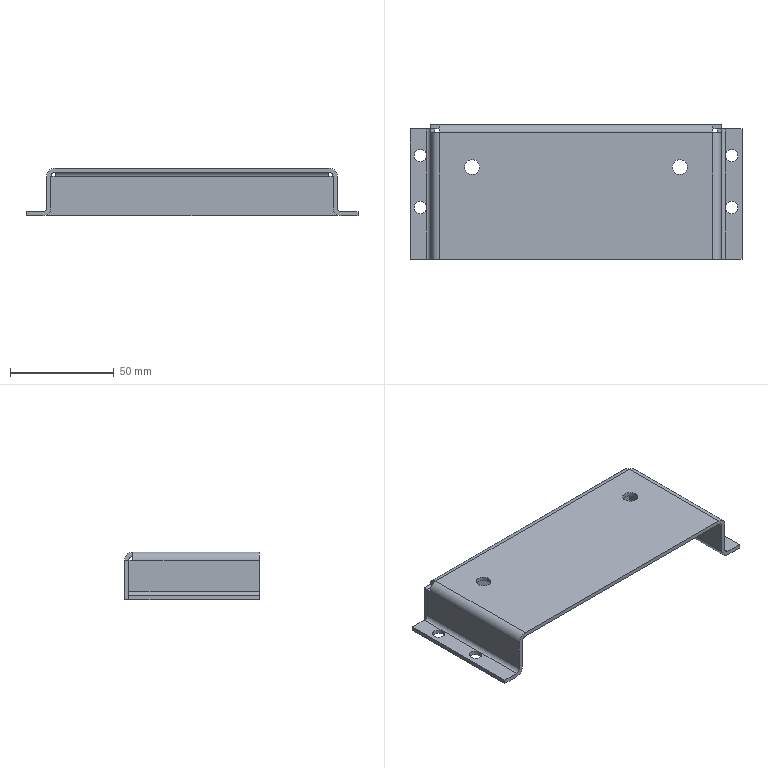Part | NX | features solid 2 | 1 solid | 50 faces | box 160 x 65 x 23 mm | volume 30401 mm3 | plane 28 | cylinder 22 | commonest cylinder face diameters 6 x8 4 x5 8 x5 7.2 x4
STEP:
#1=CARTESIAN_POINT('',(-346.,-1503.,1272.));
#2=VERTEX_POINT('',#1);
#3=CARTESIAN_POINT('',(-346.,-1503.,1274.));
#4=VERTEX_POINT('',#3);
#5=CARTESIAN_POINT('',(-346.,-1503.,1120.776));
#6=DIRECTION('',(0.,0.,1.));
#7=VECTOR('',#6,1000.);
#8=LINE('',#5,#7);
#9=EDGE_CURVE('',#2,#4,#8,.T.);
#10=ORIENTED_EDGE('',*,*,#9,.F.);
#11=CARTESIAN_POINT('',(-352.,-1503.,1272.));
#12=VERTEX_POINT('',#11);
#13=CARTESIAN_POINT('',(-349.,-1503.,1272.));
#14=DIRECTION('',(0.,0.,-1.));
#15=DIRECTION('',(1.,0.,0.));
#16=AXIS2_PLACEMENT_3D('',#13,#14,#15);
#17=CIRCLE('',#16,3.);
#18=EDGE_CURVE('',#2,#12,#17,.T.);
#19=ORIENTED_EDGE('',*,*,#18,.T.);
#20=CARTESIAN_POINT('',(-352.,-1503.,1274.));
#21=VERTEX_POINT('',#20);
#22=CARTESIAN_POINT('',(-352.,-1503.,1120.776));
#23=DIRECTION('',(0.,0.,1.));
#24=VECTOR('',#23,1000.);
#25=LINE('',#22,#24);
#26=EDGE_CURVE('',#21,#12,#25,.F.);
#27=ORIENTED_EDGE('',*,*,#26,.F.);
#28=CARTESIAN_POINT('',(-349.,-1503.,1274.));
#29=DIRECTION('',(0.,0.,-1.));
#30=DIRECTION('',(1.,0.,0.));
#31=AXIS2_PLACEMENT_3D('',#28,#29,#30);
#32=CIRCLE('',#31,3.);
#33=EDGE_CURVE('',#4,#21,#32,.T.);
#34=ORIENTED_EDGE('',*,*,#33,.F.);
#35=EDGE_LOOP('',(#10,#19,#27,#34));
#36=FACE_BOUND('',#35,.T.);
#37=CARTESIAN_POINT('',(-349.,-1503.,1120.776));
#38=DIRECTION('',(0.,0.,1.));
#39=DIRECTION('',(-1.,0.,0.));
#40=AXIS2_PLACEMENT_3D('',#37,#38,#39);
#41=CYLINDRICAL_SURFACE('',#40,3.);
#42=ADVANCED_FACE('',(#36),#41,.F.);
#43=CARTESIAN_POINT('',(-346.,-1528.,1274.));
#44=VERTEX_POINT('',#43);
#45=CARTESIAN_POINT('',(-346.,-1528.,1272.));
#46=VERTEX_POINT('',#45);
#47=CARTESIAN_POINT('',(-346.,-1528.,1120.776));
#48=DIRECTION('',(0.,0.,1.));
#49=VECTOR('',#48,1000.);
#50=LINE('',#47,#49);
#51=EDGE_CURVE('',#44,#46,#50,.F.);
#52=ORIENTED_EDGE('',*,*,#51,.T.);
#53=CARTESIAN_POINT('',(-352.,-1528.,1272.));
#54=VERTEX_POINT('',#53);
#55=CARTESIAN_POINT('',(-349.,-1528.,1272.));
#56=DIRECTION('',(0.,0.,-1.));
#57=DIRECTION('',(1.,0.,0.));
#58=AXIS2_PLACEMENT_3D('',#55,#56,#57);
#59=CIRCLE('',#58,3.);
#60=EDGE_CURVE('',#46,#54,#59,.T.);
#61=ORIENTED_EDGE('',*,*,#60,.T.);
#62=CARTESIAN_POINT('',(-352.,-1528.,1274.));
#63=VERTEX_POINT('',#62);
#64=CARTESIAN_POINT('',(-352.,-1528.,1120.776));
#65=DIRECTION('',(0.,0.,1.));
#66=VECTOR('',#65,1000.);
#67=LINE('',#64,#66);
#68=EDGE_CURVE('',#54,#63,#67,.T.);
#69=ORIENTED_EDGE('',*,*,#68,.T.);
#70=CARTESIAN_POINT('',(-349.,-1528.,1274.));
#71=DIRECTION('',(0.,0.,-1.));
#72=DIRECTION('',(1.,0.,0.));
#73=AXIS2_PLACEMENT_3D('',#70,#71,#72);
#74=CIRCLE('',#73,3.);
#75=EDGE_CURVE('',#44,#63,#74,.T.);
#76=ORIENTED_EDGE('',*,*,#75,.F.);
#77=EDGE_LOOP('',(#52,#61,#69,#76));
#78=FACE_BOUND('',#77,.T.);
#79=CARTESIAN_POINT('',(-349.,-1528.,1120.776));
#80=DIRECTION('',(0.,0.,1.));
#81=DIRECTION('',(-1.,0.,0.));
#82=AXIS2_PLACEMENT_3D('',#79,#80,#81);
#83=CYLINDRICAL_SURFACE('',#82,3.);
#84=ADVANCED_FACE('',(#78),#83,.F.);
#85=CARTESIAN_POINT('',(-496.,-1528.,1272.));
#86=VERTEX_POINT('',#85);
#87=CARTESIAN_POINT('',(-496.,-1528.,1274.));
#88=VERTEX_POINT('',#87);
#89=CARTESIAN_POINT('',(-496.,-1528.,1120.776));
#90=DIRECTION('',(0.,0.,1.));
#91=VECTOR('',#90,1000.);
#92=LINE('',#89,#91);
#93=EDGE_CURVE('',#86,#88,#92,.T.);
#94=ORIENTED_EDGE('',*,*,#93,.F.);
#95=CARTESIAN_POINT('',(-502.,-1528.,1272.));
#96=VERTEX_POINT('',#95);
#97=CARTESIAN_POINT('',(-499.,-1528.,1272.));
#98=DIRECTION('',(0.,0.,-1.));
#99=DIRECTION('',(1.,0.,0.));
#100=AXIS2_PLACEMENT_3D('',#97,#98,#99);
#101=CIRCLE('',#100,3.);
#102=EDGE_CURVE('',#86,#96,#101,.T.);
#103=ORIENTED_EDGE('',*,*,#102,.T.);
#104=CARTESIAN_POINT('',(-502.,-1528.,1274.));
#105=VERTEX_POINT('',#104);
#106=CARTESIAN_POINT('',(-502.,-1528.,1120.776));
#107=DIRECTION('',(0.,0.,1.));
#108=VECTOR('',#107,1000.);
#109=LINE('',#106,#108);
#110=EDGE_CURVE('',#105,#96,#109,.F.);
#111=ORIENTED_EDGE('',*,*,#110,.F.);
#112=CARTESIAN_POINT('',(-499.,-1528.,1274.));
#113=DIRECTION('',(0.,0.,-1.));
#114=DIRECTION('',(1.,0.,0.));
#115=AXIS2_PLACEMENT_3D('',#112,#113,#114);
#116=CIRCLE('',#115,3.);
#117=EDGE_CURVE('',#88,#105,#116,.T.);
#118=ORIENTED_EDGE('',*,*,#117,.F.);
#119=EDGE_LOOP('',(#94,#103,#111,#118));
#120=FACE_BOUND('',#119,.T.);
#121=CARTESIAN_POINT('',(-499.,-1528.,1120.776));
#122=DIRECTION('',(0.,0.,1.));
#123=DIRECTION('',(-1.,0.,0.));
#124=AXIS2_PLACEMENT_3D('',#121,#122,#123);
#125=CYLINDRICAL_SURFACE('',#124,3.);
#126=ADVANCED_FACE('',(#120),#125,.F.);
#127=CARTESIAN_POINT('',(-496.,-1503.,1274.));
#128=VERTEX_POINT('',#127);
#129=CARTESIAN_POINT('',(-496.,-1503.,1272.));
#130=VERTEX_POINT('',#129);
#131=CARTESIAN_POINT('',(-496.,-1503.,1120.776));
#132=DIRECTION('',(0.,0.,1.));
#133=VECTOR('',#132,1000.);
#134=LINE('',#131,#133);
#135=EDGE_CURVE('',#128,#130,#134,.F.);
#136=ORIENTED_EDGE('',*,*,#135,.T.);
#137=CARTESIAN_POINT('',(-502.,-1503.,1272.));
#138=VERTEX_POINT('',#137);
#139=CARTESIAN_POINT('',(-499.,-1503.,1272.));
#140=DIRECTION('',(0.,0.,-1.));
#141=DIRECTION('',(1.,0.,0.));
#142=AXIS2_PLACEMENT_3D('',#139,#140,#141);
#143=CIRCLE('',#142,3.);
#144=EDGE_CURVE('',#130,#138,#143,.T.);
#145=ORIENTED_EDGE('',*,*,#144,.T.);
#146=CARTESIAN_POINT('',(-502.,-1503.,1274.));
#147=VERTEX_POINT('',#146);
#148=CARTESIAN_POINT('',(-502.,-1503.,1120.776));
#149=DIRECTION('',(0.,0.,1.));
#150=VECTOR('',#149,1000.);
#151=LINE('',#148,#150);
#152=EDGE_CURVE('',#138,#147,#151,.T.);
#153=ORIENTED_EDGE('',*,*,#152,.T.);
#154=CARTESIAN_POINT('',(-499.,-1503.,1274.));
#155=DIRECTION('',(0.,0.,-1.));
#156=DIRECTION('',(1.,0.,0.));
#157=AXIS2_PLACEMENT_3D('',#154,#155,#156);
#158=CIRCLE('',#157,3.);
#159=EDGE_CURVE('',#128,#147,#158,.T.);
#160=ORIENTED_EDGE('',*,*,#159,.F.);
#161=EDGE_LOOP('',(#136,#145,#153,#160));
#162=FACE_BOUND('',#161,.T.);
#163=CARTESIAN_POINT('',(-499.,-1503.,1120.776));
#164=DIRECTION('',(0.,0.,1.));
#165=DIRECTION('',(-1.,0.,0.));
#166=AXIS2_PLACEMENT_3D('',#163,#164,#165);
#167=CYLINDRICAL_SURFACE('',#166,3.);
#168=ADVANCED_FACE('',(#162),#167,.F.);
#169=CARTESIAN_POINT('',(-494.,-1553.,1276.));
#170=VERTEX_POINT('',#169);
#171=CARTESIAN_POINT('',(-494.,-1490.1,1276.));
#172=VERTEX_POINT('',#171);
#173=CARTESIAN_POINT('',(-494.,-1553.,1276.));
#174=DIRECTION('',(0.,1.,0.));
#175=VECTOR('',#174,1000.);
#176=LINE('',#173,#175);
#177=EDGE_CURVE('',#170,#172,#176,.T.);
#178=ORIENTED_EDGE('',*,*,#177,.T.);
#179=CARTESIAN_POINT('',(-496.,-1490.1,1274.));
#180=VERTEX_POINT('',#179);
#181=CARTESIAN_POINT('',(-496.,-1490.1,1276.));
#182=DIRECTION('',(0.,1.,0.));
#183=DIRECTION('',(0.,0.,-1.));
#184=AXIS2_PLACEMENT_3D('',#181,#182,#183);
#185=CIRCLE('',#184,2.);
#186=EDGE_CURVE('',#172,#180,#185,.T.);
#187=ORIENTED_EDGE('',*,*,#186,.T.);
#188=CARTESIAN_POINT('',(-496.,-1490.1,1274.));
#189=DIRECTION('',(0.,-1.,0.));
#190=VECTOR('',#189,1000.);
#191=LINE('',#188,#190);
#192=EDGE_CURVE('',#180,#128,#191,.T.);
#193=ORIENTED_EDGE('',*,*,#192,.T.);
#194=CARTESIAN_POINT('',(-496.,-1490.1,1274.));
#195=DIRECTION('',(0.,-1.,0.));
#196=VECTOR('',#195,1000.);
#197=LINE('',#194,#196);
#198=EDGE_CURVE('',#128,#88,#197,.T.);
#199=ORIENTED_EDGE('',*,*,#198,.T.);
#200=CARTESIAN_POINT('',(-496.,-1553.,1274.));
#201=VERTEX_POINT('',#200);
#202=CARTESIAN_POINT('',(-496.,-1490.1,1274.));
#203=DIRECTION('',(0.,-1.,0.));
#204=VECTOR('',#203,1000.);
#205=LINE('',#202,#204);
#206=EDGE_CURVE('',#88,#201,#205,.T.);
#207=ORIENTED_EDGE('',*,*,#206,.T.);
#208=CARTESIAN_POINT('',(-496.,-1553.,1276.));
#209=DIRECTION('',(0.,1.,0.));
#210=DIRECTION('',(0.,0.,-1.));
#211=AXIS2_PLACEMENT_3D('',#208,#209,#210);
#212=CIRCLE('',#211,2.);
#213=EDGE_CURVE('',#170,#201,#212,.T.);
#214=ORIENTED_EDGE('',*,*,#213,.F.);
#215=EDGE_LOOP('',(#178,#187,#193,#199,#207,#214));
#216=FACE_BOUND('',#215,.T.);
#217=CARTESIAN_POINT('',(-496.,-1553.,1276.));
#218=DIRECTION('',(0.,1.,0.));
#219=DIRECTION('',(-1.,0.,0.));
#220=AXIS2_PLACEMENT_3D('',#217,#218,#219);
#221=CYLINDRICAL_SURFACE('',#220,2.);
#222=ADVANCED_FACE('',(#216),#221,.F.);
#223=CARTESIAN_POINT('',(-492.,-1553.,1276.));
#224=VERTEX_POINT('',#223);
#225=CARTESIAN_POINT('',(-492.,-1490.1,1276.));
#226=VERTEX_POINT('',#225);
#227=CARTESIAN_POINT('',(-492.,-1553.,1276.));
#228=DIRECTION('',(0.,1.,0.));
#229=VECTOR('',#228,1000.);
#230=LINE('',#227,#229);
#231=EDGE_CURVE('',#224,#226,#230,.T.);
#232=ORIENTED_EDGE('',*,*,#231,.F.);
#233=CARTESIAN_POINT('',(-496.,-1553.,1272.));
#234=VERTEX_POINT('',#233);
#235=CARTESIAN_POINT('',(-496.,-1553.,1276.));
#236=DIRECTION('',(0.,1.,0.));
#237=DIRECTION('',(-1.,0.,0.));
#238=AXIS2_PLACEMENT_3D('',#235,#236,#237);
#239=CIRCLE('',#238,4.);
#240=EDGE_CURVE('',#224,#234,#239,.T.);
#241=ORIENTED_EDGE('',*,*,#240,.T.);
#242=CARTESIAN_POINT('',(-496.,-1490.1,1272.));
#243=DIRECTION('',(0.,-1.,0.));
#244=VECTOR('',#243,1000.);
#245=LINE('',#242,#244);
#246=EDGE_CURVE('',#86,#234,#245,.T.);
#247=ORIENTED_EDGE('',*,*,#246,.F.);
#248=CARTESIAN_POINT('',(-496.,-1490.1,1272.));
#249=DIRECTION('',(0.,-1.,0.));
#250=VECTOR('',#249,1000.);
#251=LINE('',#248,#250);
#252=EDGE_CURVE('',#130,#86,#251,.T.);
#253=ORIENTED_EDGE('',*,*,#252,.F.);
#254=CARTESIAN_POINT('',(-496.,-1490.1,1272.));
#255=VERTEX_POINT('',#254);
#256=CARTESIAN_POINT('',(-496.,-1490.1,1272.));
#257=DIRECTION('',(0.,-1.,0.));
#258=VECTOR('',#257,1000.);
#259=LINE('',#256,#258);
#260=EDGE_CURVE('',#255,#130,#259,.T.);
#261=ORIENTED_EDGE('',*,*,#260,.F.);
#262=CARTESIAN_POINT('',(-496.,-1490.1,1276.));
#263=DIRECTION('',(0.,1.,0.));
#264=DIRECTION('',(-1.,0.,0.));
#265=AXIS2_PLACEMENT_3D('',#262,#263,#264);
#266=CIRCLE('',#265,4.);
#267=EDGE_CURVE('',#226,#255,#266,.T.);
#268=ORIENTED_EDGE('',*,*,#267,.F.);
#269=EDGE_LOOP('',(#232,#241,#247,#253,#261,#268));
#270=FACE_BOUND('',#269,.T.);
#271=CARTESIAN_POINT('',(-496.,-1553.,1276.));
#272=DIRECTION('',(0.,1.,0.));
#273=DIRECTION('',(-1.,0.,0.));
#274=AXIS2_PLACEMENT_3D('',#271,#272,#273);
#275=CYLINDRICAL_SURFACE('',#274,4.);
#276=ADVANCED_FACE('',(#270),#275,.T.);
#277=CARTESIAN_POINT('',(-504.,-1553.,1274.));
#278=VERTEX_POINT('',#277);
#279=CARTESIAN_POINT('',(-504.,-1490.1,1274.));
#280=VERTEX_POINT('',#279);
#281=CARTESIAN_POINT('',(-504.,-1553.,1274.));
#282=DIRECTION('',(0.,1.,0.));
#283=VECTOR('',#282,1000.);
#284=LINE('',#281,#283);
#285=EDGE_CURVE('',#278,#280,#284,.T.);
#286=ORIENTED_EDGE('',*,*,#285,.T.);
#287=CARTESIAN_POINT('',(-504.,-1490.1,1272.));
#288=VERTEX_POINT('',#287);
#289=CARTESIAN_POINT('',(-504.,-1490.1,1272.));
#290=DIRECTION('',(0.,0.,1.));
#291=VECTOR('',#290,1000.);
#292=LINE('',#289,#291);
#293=EDGE_CURVE('',#288,#280,#292,.T.);
#294=ORIENTED_EDGE('',*,*,#293,.F.);
#295=CARTESIAN_POINT('',(-504.,-1553.,1272.));
#296=VERTEX_POINT('',#295);
#297=CARTESIAN_POINT('',(-504.,-1553.,1272.));
#298=DIRECTION('',(0.,1.,0.));
#299=VECTOR('',#298,1000.);
#300=LINE('',#297,#299);
#301=EDGE_CURVE('',#296,#288,#300,.T.);
#302=ORIENTED_EDGE('',*,*,#301,.F.);
#303=CARTESIAN_POINT('',(-504.,-1553.,1272.));
#304=DIRECTION('',(0.,0.,1.));
#305=VECTOR('',#304,1000.);
#306=LINE('',#303,#305);
#307=EDGE_CURVE('',#296,#278,#306,.T.);
#308=ORIENTED_EDGE('',*,*,#307,.T.);
#309=EDGE_LOOP('',(#286,#294,#302,#308));
#310=FACE_BOUND('',#309,.T.);
#311=CARTESIAN_POINT('',(-504.,-1553.,1272.));
#312=DIRECTION('',(1.,0.,0.));
#313=DIRECTION('',(0.,0.,-1.));
#314=AXIS2_PLACEMENT_3D('',#311,#312,#313);
#315=PLANE('',#314);
#316=ADVANCED_FACE('',(#310),#315,.F.);
#317=ORIENTED_EDGE('',*,*,#206,.F.);
#318=ORIENTED_EDGE('',*,*,#117,.T.);
#319=CARTESIAN_POINT('',(-499.,-1528.,1274.));
#320=DIRECTION('',(0.,0.,-1.));
#321=DIRECTION('',(1.,0.,0.));
#322=AXIS2_PLACEMENT_3D('',#319,#320,#321);
#323=CIRCLE('',#322,3.);
#324=EDGE_CURVE('',#105,#88,#323,.T.);
#325=ORIENTED_EDGE('',*,*,#324,.T.);
#326=ORIENTED_EDGE('',*,*,#198,.F.);
#327=ORIENTED_EDGE('',*,*,#159,.T.);
#328=CARTESIAN_POINT('',(-499.,-1503.,1274.));
#329=DIRECTION('',(0.,0.,-1.));
#330=DIRECTION('',(1.,0.,0.));
#331=AXIS2_PLACEMENT_3D('',#328,#329,#330);
#332=CIRCLE('',#331,3.);
#333=EDGE_CURVE('',#147,#128,#332,.T.);
#334=ORIENTED_EDGE('',*,*,#333,.T.);
#335=ORIENTED_EDGE('',*,*,#192,.F.);
#336=CARTESIAN_POINT('',(-493.722,-1490.1,1274.));
#337=DIRECTION('',(1.,0.,0.));
#338=VECTOR('',#337,1000.);
#339=LINE('',#336,#338);
#340=EDGE_CURVE('',#280,#180,#339,.T.);
#341=ORIENTED_EDGE('',*,*,#340,.F.);
#342=ORIENTED_EDGE('',*,*,#285,.F.);
#343=CARTESIAN_POINT('',(-493.722,-1553.,1274.));
#344=DIRECTION('',(-1.,0.,0.));
#345=VECTOR('',#344,1000.);
#346=LINE('',#343,#345);
#347=EDGE_CURVE('',#201,#278,#346,.T.);
#348=ORIENTED_EDGE('',*,*,#347,.F.);
#349=EDGE_LOOP('',(#317,#318,#325,#326,#327,#334,#335,#341,#342,#348));
#350=FACE_BOUND('',#349,.T.);
#351=CARTESIAN_POINT('',(-1166.5,-2145.,1274.));
#352=DIRECTION('',(0.,0.,-1.));
#353=DIRECTION('',(-1.,0.,0.));
#354=AXIS2_PLACEMENT_3D('',#351,#352,#353);
#355=PLANE('',#354);
#356=ADVANCED_FACE('',(#350),#355,.F.);
#357=ORIENTED_EDGE('',*,*,#252,.T.);
#358=CARTESIAN_POINT('',(-499.,-1528.,1272.));
#359=DIRECTION('',(0.,0.,-1.));
#360=DIRECTION('',(1.,0.,0.));
#361=AXIS2_PLACEMENT_3D('',#358,#359,#360);
#362=CIRCLE('',#361,3.);
#363=EDGE_CURVE('',#96,#86,#362,.T.);
#364=ORIENTED_EDGE('',*,*,#363,.F.);
#365=ORIENTED_EDGE('',*,*,#102,.F.);
#366=ORIENTED_EDGE('',*,*,#246,.T.);
#367=CARTESIAN_POINT('',(-493.722,-1553.,1272.));
#368=DIRECTION('',(-1.,0.,0.));
#369=VECTOR('',#368,1000.);
#370=LINE('',#367,#369);
#371=EDGE_CURVE('',#234,#296,#370,.T.);
#372=ORIENTED_EDGE('',*,*,#371,.T.);
#373=ORIENTED_EDGE('',*,*,#301,.T.);
#374=CARTESIAN_POINT('',(-493.722,-1490.1,1272.));
#375=DIRECTION('',(1.,0.,0.));
#376=VECTOR('',#375,1000.);
#377=LINE('',#374,#376);
#378=EDGE_CURVE('',#288,#255,#377,.T.);
#379=ORIENTED_EDGE('',*,*,#378,.T.);
#380=ORIENTED_EDGE('',*,*,#260,.T.);
#381=CARTESIAN_POINT('',(-499.,-1503.,1272.));
#382=DIRECTION('',(0.,0.,-1.));
#383=DIRECTION('',(1.,0.,0.));
#384=AXIS2_PLACEMENT_3D('',#381,#382,#383);
#385=CIRCLE('',#384,3.);
#386=EDGE_CURVE('',#138,#130,#385,.T.);
#387=ORIENTED_EDGE('',*,*,#386,.F.);
#388=ORIENTED_EDGE('',*,*,#144,.F.);
#389=EDGE_LOOP('',(#357,#364,#365,#366,#372,#373,#379,#380,#387,#388));
#390=FACE_BOUND('',#389,.T.);
#391=CARTESIAN_POINT('',(-1166.5,-2145.,1272.));
#392=DIRECTION('',(0.,0.,-1.));
#393=DIRECTION('',(-1.,0.,0.));
#394=AXIS2_PLACEMENT_3D('',#391,#392,#393);
#395=PLANE('',#394);
#396=ADVANCED_FACE('',(#390),#395,.T.);
#397=CARTESIAN_POINT('',(-354.,-1490.1,1276.));
#398=VERTEX_POINT('',#397);
#399=CARTESIAN_POINT('',(-354.,-1553.,1276.));
#400=VERTEX_POINT('',#399);
#401=CARTESIAN_POINT('',(-354.,-1490.1,1276.));
#402=DIRECTION('',(0.,-1.,0.));
#403=VECTOR('',#402,1000.);
#404=LINE('',#401,#403);
#405=EDGE_CURVE('',#398,#400,#404,.T.);
#406=ORIENTED_EDGE('',*,*,#405,.T.);
#407=CARTESIAN_POINT('',(-352.,-1553.,1274.));
#408=VERTEX_POINT('',#407);
#409=CARTESIAN_POINT('',(-352.,-1553.,1276.));
#410=DIRECTION('',(0.,-1.,0.));
#411=DIRECTION('',(1.,0.,0.));
#412=AXIS2_PLACEMENT_3D('',#409,#410,#411);
#413=CIRCLE('',#412,2.);
#414=EDGE_CURVE('',#400,#408,#413,.T.);
#415=ORIENTED_EDGE('',*,*,#414,.T.);
#416=CARTESIAN_POINT('',(-352.,-1553.,1274.));
#417=DIRECTION('',(0.,1.,0.));
#418=VECTOR('',#417,1000.);
#419=LINE('',#416,#418);
#420=EDGE_CURVE('',#408,#63,#419,.T.);
#421=ORIENTED_EDGE('',*,*,#420,.T.);
#422=CARTESIAN_POINT('',(-352.,-1553.,1274.));
#423=DIRECTION('',(0.,1.,0.));
#424=VECTOR('',#423,1000.);
#425=LINE('',#422,#424);
#426=EDGE_CURVE('',#63,#21,#425,.T.);
#427=ORIENTED_EDGE('',*,*,#426,.T.);
#428=CARTESIAN_POINT('',(-352.,-1490.1,1274.));
#429=VERTEX_POINT('',#428);
#430=CARTESIAN_POINT('',(-352.,-1553.,1274.));
#431=DIRECTION('',(0.,1.,0.));
#432=VECTOR('',#431,1000.);
#433=LINE('',#430,#432);
#434=EDGE_CURVE('',#21,#429,#433,.T.);
#435=ORIENTED_EDGE('',*,*,#434,.T.);
#436=CARTESIAN_POINT('',(-352.,-1490.1,1276.));
#437=DIRECTION('',(0.,-1.,0.));
#438=DIRECTION('',(1.,0.,0.));
#439=AXIS2_PLACEMENT_3D('',#436,#437,#438);
#440=CIRCLE('',#439,2.);
#441=EDGE_CURVE('',#398,#429,#440,.T.);
#442=ORIENTED_EDGE('',*,*,#441,.F.);
#443=EDGE_LOOP('',(#406,#415,#421,#427,#435,#442));
#444=FACE_BOUND('',#443,.T.);
#445=CARTESIAN_POINT('',(-352.,-1490.1,1276.));
#446=DIRECTION('',(0.,-1.,0.));
#447=DIRECTION('',(1.,0.,0.));
#448=AXIS2_PLACEMENT_3D('',#445,#446,#447);
#449=CYLINDRICAL_SURFACE('',#448,2.);
#450=ADVANCED_FACE('',(#444),#449,.F.);
#451=CARTESIAN_POINT('',(-356.,-1490.1,1276.));
#452=VERTEX_POINT('',#451);
#453=CARTESIAN_POINT('',(-356.,-1553.,1276.));
#454=VERTEX_POINT('',#453);
#455=CARTESIAN_POINT('',(-356.,-1490.1,1276.));
#456=DIRECTION('',(0.,-1.,0.));
#457=VECTOR('',#456,1000.);
#458=LINE('',#455,#457);
#459=EDGE_CURVE('',#452,#454,#458,.T.);
#460=ORIENTED_EDGE('',*,*,#459,.F.);
#461=CARTESIAN_POINT('',(-352.,-1490.1,1272.));
#462=VERTEX_POINT('',#461);
#463=CARTESIAN_POINT('',(-352.,-1490.1,1276.));
#464=DIRECTION('',(0.,-1.,0.));
#465=DIRECTION('',(1.,0.,0.));
#466=AXIS2_PLACEMENT_3D('',#463,#464,#465);
#467=CIRCLE('',#466,4.);
#468=EDGE_CURVE('',#452,#462,#467,.T.);
#469=ORIENTED_EDGE('',*,*,#468,.T.);
#470=CARTESIAN_POINT('',(-352.,-1553.,1272.));
#471=DIRECTION('',(0.,1.,0.));
#472=VECTOR('',#471,1000.);
#473=LINE('',#470,#472);
#474=EDGE_CURVE('',#12,#462,#473,.T.);
#475=ORIENTED_EDGE('',*,*,#474,.F.);
#476=CARTESIAN_POINT('',(-352.,-1553.,1272.));
#477=DIRECTION('',(0.,1.,0.));
#478=VECTOR('',#477,1000.);
#479=LINE('',#476,#478);
#480=EDGE_CURVE('',#54,#12,#479,.T.);
#481=ORIENTED_EDGE('',*,*,#480,.F.);
#482=CARTESIAN_POINT('',(-352.,-1553.,1272.));
#483=VERTEX_POINT('',#482);
#484=CARTESIAN_POINT('',(-352.,-1553.,1272.));
#485=DIRECTION('',(0.,1.,0.));
#486=VECTOR('',#485,1000.);
#487=LINE('',#484,#486);
#488=EDGE_CURVE('',#483,#54,#487,.T.);
#489=ORIENTED_EDGE('',*,*,#488,.F.);
#490=CARTESIAN_POINT('',(-352.,-1553.,1276.));
#491=DIRECTION('',(0.,-1.,0.));
#492=DIRECTION('',(1.,0.,0.));
#493=AXIS2_PLACEMENT_3D('',#490,#491,#492);
#494=CIRCLE('',#493,4.);
#495=EDGE_CURVE('',#454,#483,#494,.T.);
#496=ORIENTED_EDGE('',*,*,#495,.F.);
#497=EDGE_LOOP('',(#460,#469,#475,#481,#489,#496));
#498=FACE_BOUND('',#497,.T.);
#499=CARTESIAN_POINT('',(-352.,-1490.1,1276.));
#500=DIRECTION('',(0.,-1.,0.));
#501=DIRECTION('',(1.,0.,0.));
#502=AXIS2_PLACEMENT_3D('',#499,#500,#501);
#503=CYLINDRICAL_SURFACE('',#502,4.);
#504=ADVANCED_FACE('',(#498),#503,.T.);
#505=CARTESIAN_POINT('',(-344.,-1490.1,1274.));
#506=VERTEX_POINT('',#505);
#507=CARTESIAN_POINT('',(-344.,-1553.,1274.));
#508=VERTEX_POINT('',#507);
#509=CARTESIAN_POINT('',(-344.,-1490.1,1274.));
#510=DIRECTION('',(0.,-1.,0.));
#511=VECTOR('',#510,1000.);
#512=LINE('',#509,#511);
#513=EDGE_CURVE('',#506,#508,#512,.T.);
#514=ORIENTED_EDGE('',*,*,#513,.T.);
#515=CARTESIAN_POINT('',(-344.,-1553.,1272.));
#516=VERTEX_POINT('',#515);
#517=CARTESIAN_POINT('',(-344.,-1553.,1272.));
#518=DIRECTION('',(0.,0.,1.));
#519=VECTOR('',#518,1000.);
#520=LINE('',#517,#519);
#521=EDGE_CURVE('',#516,#508,#520,.T.);
#522=ORIENTED_EDGE('',*,*,#521,.F.);
#523=CARTESIAN_POINT('',(-344.,-1490.1,1272.));
#524=VERTEX_POINT('',#523);
#525=CARTESIAN_POINT('',(-344.,-1490.1,1272.));
#526=DIRECTION('',(0.,-1.,0.));
#527=VECTOR('',#526,1000.);
#528=LINE('',#525,#527);
#529=EDGE_CURVE('',#524,#516,#528,.T.);
#530=ORIENTED_EDGE('',*,*,#529,.F.);
#531=CARTESIAN_POINT('',(-344.,-1490.1,1272.));
#532=DIRECTION('',(0.,0.,1.));
#533=VECTOR('',#532,1000.);
#534=LINE('',#531,#533);
#535=EDGE_CURVE('',#524,#506,#534,.T.);
#536=ORIENTED_EDGE('',*,*,#535,.T.);
#537=EDGE_LOOP('',(#514,#522,#530,#536));
#538=FACE_BOUND('',#537,.T.);
#539=CARTESIAN_POINT('',(-344.,-1490.1,1272.));
#540=DIRECTION('',(-1.,0.,0.));
#541=DIRECTION('',(0.,0.,1.));
#542=AXIS2_PLACEMENT_3D('',#539,#540,#541);
#543=PLANE('',#542);
#544=ADVANCED_FACE('',(#538),#543,.F.);
#545=ORIENTED_EDGE('',*,*,#434,.F.);
#546=CARTESIAN_POINT('',(-349.,-1503.,1274.));
#547=DIRECTION('',(0.,0.,-1.));
#548=DIRECTION('',(1.,0.,0.));
#549=AXIS2_PLACEMENT_3D('',#546,#547,#548);
#550=CIRCLE('',#549,3.);
#551=EDGE_CURVE('',#21,#4,#550,.T.);
#552=ORIENTED_EDGE('',*,*,#551,.T.);
#553=ORIENTED_EDGE('',*,*,#33,.T.);
#554=ORIENTED_EDGE('',*,*,#426,.F.);
#555=CARTESIAN_POINT('',(-349.,-1528.,1274.));
#556=DIRECTION('',(0.,0.,-1.));
#557=DIRECTION('',(1.,0.,0.));
#558=AXIS2_PLACEMENT_3D('',#555,#556,#557);
#559=CIRCLE('',#558,3.);
#560=EDGE_CURVE('',#63,#44,#559,.T.);
#561=ORIENTED_EDGE('',*,*,#560,.T.);
#562=ORIENTED_EDGE('',*,*,#75,.T.);
#563=ORIENTED_EDGE('',*,*,#420,.F.);
#564=CARTESIAN_POINT('',(-354.278,-1553.,1274.));
#565=DIRECTION('',(-1.,0.,0.));
#566=VECTOR('',#565,1000.);
#567=LINE('',#564,#566);
#568=EDGE_CURVE('',#508,#408,#567,.T.);
#569=ORIENTED_EDGE('',*,*,#568,.F.);
#570=ORIENTED_EDGE('',*,*,#513,.F.);
#571=CARTESIAN_POINT('',(-354.278,-1490.1,1274.));
#572=DIRECTION('',(1.,0.,0.));
#573=VECTOR('',#572,1000.);
#574=LINE('',#571,#573);
#575=EDGE_CURVE('',#429,#506,#574,.T.);
#576=ORIENTED_EDGE('',*,*,#575,.F.);
#577=EDGE_LOOP('',(#545,#552,#553,#554,#561,#562,#563,#569,#570,#576));
#578=FACE_BOUND('',#577,.T.);
#579=CARTESIAN_POINT('',(-1166.5,-2145.,1274.));
#580=DIRECTION('',(0.,0.,-1.));
#581=DIRECTION('',(0.,-1.,0.));
#582=AXIS2_PLACEMENT_3D('',#579,#580,#581);
#583=PLANE('',#582);
#584=ADVANCED_FACE('',(#578),#583,.F.);
#585=ORIENTED_EDGE('',*,*,#480,.T.);
#586=ORIENTED_EDGE('',*,*,#18,.F.);
#587=CARTESIAN_POINT('',(-349.,-1503.,1272.));
#588=DIRECTION('',(0.,0.,-1.));
#589=DIRECTION('',(1.,0.,0.));
#590=AXIS2_PLACEMENT_3D('',#587,#588,#589);
#591=CIRCLE('',#590,3.);
#592=EDGE_CURVE('',#12,#2,#591,.T.);
#593=ORIENTED_EDGE('',*,*,#592,.F.);
#594=ORIENTED_EDGE('',*,*,#474,.T.);
#595=CARTESIAN_POINT('',(-354.278,-1490.1,1272.));
#596=DIRECTION('',(1.,0.,0.));
#597=VECTOR('',#596,1000.);
#598=LINE('',#595,#597);
#599=EDGE_CURVE('',#462,#524,#598,.T.);
#600=ORIENTED_EDGE('',*,*,#599,.T.);
#601=ORIENTED_EDGE('',*,*,#529,.T.);
#602=CARTESIAN_POINT('',(-354.278,-1553.,1272.));
#603=DIRECTION('',(-1.,0.,0.));
#604=VECTOR('',#603,1000.);
#605=LINE('',#602,#604);
#606=EDGE_CURVE('',#516,#483,#605,.T.);
#607=ORIENTED_EDGE('',*,*,#606,.T.);
#608=ORIENTED_EDGE('',*,*,#488,.T.);
#609=ORIENTED_EDGE('',*,*,#60,.F.);
#610=CARTESIAN_POINT('',(-349.,-1528.,1272.));
#611=DIRECTION('',(0.,0.,-1.));
#612=DIRECTION('',(1.,0.,0.));
#613=AXIS2_PLACEMENT_3D('',#610,#611,#612);
#614=CIRCLE('',#613,3.);
#615=EDGE_CURVE('',#54,#46,#614,.T.);
#616=ORIENTED_EDGE('',*,*,#615,.F.);
#617=EDGE_LOOP('',(#585,#586,#593,#594,#600,#601,#607,#608,#609,#616));
#618=FACE_BOUND('',#617,.T.);
#619=CARTESIAN_POINT('',(-1166.5,-2145.,1272.));
#620=DIRECTION('',(0.,0.,-1.));
#621=DIRECTION('',(0.,-1.,0.));
#622=AXIS2_PLACEMENT_3D('',#619,#620,#621);
#623=PLANE('',#622);
#624=ADVANCED_FACE('',(#618),#623,.T.);
#625=CARTESIAN_POINT('',(-370.4,-1508.5,1295.));
#626=VERTEX_POINT('',#625);
#627=CARTESIAN_POINT('',(-370.4,-1508.5,1293.));
#628=VERTEX_POINT('',#627);
#629=CARTESIAN_POINT('',(-370.4,-1508.5,1138.942));
#630=DIRECTION('',(0.,0.,1.));
#631=VECTOR('',#630,1000.);
#632=LINE('',#629,#631);
#633=EDGE_CURVE('',#626,#628,#632,.F.);
#634=ORIENTED_EDGE('',*,*,#633,.T.);
#635=CARTESIAN_POINT('',(-377.6,-1508.5,1293.));
#636=VERTEX_POINT('',#635);
#637=CARTESIAN_POINT('',(-374.,-1508.5,1293.));
#638=DIRECTION('',(0.,0.,-1.));
#639=DIRECTION('',(1.,0.,0.));
#640=AXIS2_PLACEMENT_3D('',#637,#638,#639);
#641=CIRCLE('',#640,3.6);
#642=EDGE_CURVE('',#628,#636,#641,.T.);
#643=ORIENTED_EDGE('',*,*,#642,.T.);
#644=CARTESIAN_POINT('',(-377.6,-1508.5,1295.));
#645=VERTEX_POINT('',#644);
#646=CARTESIAN_POINT('',(-377.6,-1508.5,1138.942));
#647=DIRECTION('',(0.,0.,1.));
#648=VECTOR('',#647,1000.);
#649=LINE('',#646,#648);
#650=EDGE_CURVE('',#636,#645,#649,.T.);
#651=ORIENTED_EDGE('',*,*,#650,.T.);
#652=CARTESIAN_POINT('',(-374.,-1508.5,1295.));
#653=DIRECTION('',(0.,0.,1.));
#654=DIRECTION('',(-1.,0.,0.));
#655=AXIS2_PLACEMENT_3D('',#652,#653,#654);
#656=CIRCLE('',#655,3.6);
#657=EDGE_CURVE('',#645,#626,#656,.T.);
#658=ORIENTED_EDGE('',*,*,#657,.T.);
#659=EDGE_LOOP('',(#634,#643,#651,#658));
#660=FACE_BOUND('',#659,.T.);
#661=CARTESIAN_POINT('',(-374.,-1508.5,1138.942));
#662=DIRECTION('',(0.,0.,1.));
#663=DIRECTION('',(-1.,0.,0.));
#664=AXIS2_PLACEMENT_3D('',#661,#662,#663);
#665=CYLINDRICAL_SURFACE('',#664,3.6);
#666=ADVANCED_FACE('',(#660),#665,.F.);
#667=CARTESIAN_POINT('',(-470.4,-1508.5,1293.));
#668=VERTEX_POINT('',#667);
#669=CARTESIAN_POINT('',(-470.4,-1508.5,1295.));
#670=VERTEX_POINT('',#669);
#671=CARTESIAN_POINT('',(-470.4,-1508.5,1138.942));
#672=DIRECTION('',(0.,0.,1.));
#673=VECTOR('',#672,1000.);
#674=LINE('',#671,#673);
#675=EDGE_CURVE('',#668,#670,#674,.T.);
#676=ORIENTED_EDGE('',*,*,#675,.F.);
#677=CARTESIAN_POINT('',(-477.6,-1508.5,1293.));
#678=VERTEX_POINT('',#677);
#679=CARTESIAN_POINT('',(-474.,-1508.5,1293.));
#680=DIRECTION('',(0.,0.,-1.));
#681=DIRECTION('',(1.,0.,0.));
#682=AXIS2_PLACEMENT_3D('',#679,#680,#681);
#683=CIRCLE('',#682,3.6);
#684=EDGE_CURVE('',#668,#678,#683,.T.);
#685=ORIENTED_EDGE('',*,*,#684,.T.);
#686=CARTESIAN_POINT('',(-477.6,-1508.5,1295.));
#687=VERTEX_POINT('',#686);
#688=CARTESIAN_POINT('',(-477.6,-1508.5,1138.942));
#689=DIRECTION('',(0.,0.,1.));
#690=VECTOR('',#689,1000.);
#691=LINE('',#688,#690);
#692=EDGE_CURVE('',#687,#678,#691,.F.);
#693=ORIENTED_EDGE('',*,*,#692,.F.);
#694=CARTESIAN_POINT('',(-474.,-1508.5,1295.));
#695=DIRECTION('',(0.,0.,1.));
#696=DIRECTION('',(-1.,0.,0.));
#697=AXIS2_PLACEMENT_3D('',#694,#695,#696);
#698=CIRCLE('',#697,3.6);
#699=EDGE_CURVE('',#687,#670,#698,.T.);
#700=ORIENTED_EDGE('',*,*,#699,.T.);
#701=EDGE_LOOP('',(#676,#685,#693,#700));
#702=FACE_BOUND('',#701,.T.);
#703=CARTESIAN_POINT('',(-474.,-1508.5,1138.942));
#704=DIRECTION('',(0.,0.,1.));
#705=DIRECTION('',(-1.,0.,0.));
#706=AXIS2_PLACEMENT_3D('',#703,#704,#705);
#707=CYLINDRICAL_SURFACE('',#706,3.6);
#708=ADVANCED_FACE('',(#702),#707,.F.);
#709=CARTESIAN_POINT('',(-494.,-1490.,1291.));
#710=VERTEX_POINT('',#709);
#711=CARTESIAN_POINT('',(-494.,-1490.,1272.));
#712=VERTEX_POINT('',#711);
#713=CARTESIAN_POINT('',(-494.,-1490.,1295.));
#714=DIRECTION('',(0.,0.,-1.));
#715=VECTOR('',#714,1000.);
#716=LINE('',#713,#715);
#717=EDGE_CURVE('',#710,#712,#716,.T.);
#718=ORIENTED_EDGE('',*,*,#717,.T.);
#719=CARTESIAN_POINT('',(-354.,-1490.,1272.));
#720=VERTEX_POINT('',#719);
#721=CARTESIAN_POINT('',(44.,-1490.,1272.));
#722=DIRECTION('',(-1.,0.,0.));
#723=VECTOR('',#722,1000.);
#724=LINE('',#721,#723);
#725=EDGE_CURVE('',#720,#712,#724,.T.);
#726=ORIENTED_EDGE('',*,*,#725,.F.);
#727=CARTESIAN_POINT('',(-354.,-1490.,1291.));
#728=VERTEX_POINT('',#727);
#729=CARTESIAN_POINT('',(-354.,-1490.,1295.));
#730=DIRECTION('',(0.,0.,-1.));
#731=VECTOR('',#730,1000.);
#732=LINE('',#729,#731);
#733=EDGE_CURVE('',#728,#720,#732,.T.);
#734=ORIENTED_EDGE('',*,*,#733,.F.);
#735=CARTESIAN_POINT('',(-358.,-1490.,1291.));
#736=VERTEX_POINT('',#735);
#737=CARTESIAN_POINT('',(44.,-1490.,1291.));
#738=DIRECTION('',(-1.,0.,0.));
#739=VECTOR('',#738,1000.);
#740=LINE('',#737,#739);
#741=EDGE_CURVE('',#728,#736,#740,.T.);
#742=ORIENTED_EDGE('',*,*,#741,.T.);
#743=CARTESIAN_POINT('',(-490.,-1490.,1291.));
#744=VERTEX_POINT('',#743);
#745=CARTESIAN_POINT('',(44.,-1490.,1291.));
#746=DIRECTION('',(-1.,0.,0.));
#747=VECTOR('',#746,1000.);
#748=LINE('',#745,#747);
#749=EDGE_CURVE('',#736,#744,#748,.T.);
#750=ORIENTED_EDGE('',*,*,#749,.T.);
#751=CARTESIAN_POINT('',(44.,-1490.,1291.));
#752=DIRECTION('',(-1.,0.,0.));
#753=VECTOR('',#752,1000.);
#754=LINE('',#751,#753);
#755=EDGE_CURVE('',#744,#710,#754,.T.);
#756=ORIENTED_EDGE('',*,*,#755,.T.);
#757=EDGE_LOOP('',(#718,#726,#734,#742,#750,#756));
#758=FACE_BOUND('',#757,.T.);
#759=CARTESIAN_POINT('',(44.,-1490.,1295.));
#760=DIRECTION('',(0.,1.,0.));
#761=DIRECTION('',(0.,0.,-1.));
#762=AXIS2_PLACEMENT_3D('',#759,#760,#761);
#763=PLANE('',#762);
#764=ADVANCED_FACE('',(#758),#763,.F.);
#765=CARTESIAN_POINT('',(-354.,-1488.,1291.));
#766=VERTEX_POINT('',#765);
#767=CARTESIAN_POINT('',(-354.,-1488.,1291.));
#768=DIRECTION('',(0.,1.,0.));
#769=VECTOR('',#768,1000.);
#770=LINE('',#767,#769);
#771=EDGE_CURVE('',#728,#766,#770,.T.);
#772=ORIENTED_EDGE('',*,*,#771,.F.);
#773=ORIENTED_EDGE('',*,*,#733,.T.);
#774=CARTESIAN_POINT('',(-354.,-1488.,1272.));
#775=VERTEX_POINT('',#774);
#776=CARTESIAN_POINT('',(-354.,-1488.,1272.));
#777=DIRECTION('',(0.,1.,0.));
#778=VECTOR('',#777,1000.);
#779=LINE('',#776,#778);
#780=EDGE_CURVE('',#720,#775,#779,.T.);
#781=ORIENTED_EDGE('',*,*,#780,.T.);
#782=CARTESIAN_POINT('',(-354.,-1488.,1291.));
#783=DIRECTION('',(0.,0.,-1.));
#784=VECTOR('',#783,1000.);
#785=LINE('',#782,#784);
#786=EDGE_CURVE('',#766,#775,#785,.T.);
#787=ORIENTED_EDGE('',*,*,#786,.F.);
#788=EDGE_LOOP('',(#772,#773,#781,#787));
#789=FACE_BOUND('',#788,.T.);
#790=CARTESIAN_POINT('',(-354.,-1488.,1291.));
#791=DIRECTION('',(1.,0.,0.));
#792=DIRECTION('',(0.,0.,-1.));
#793=AXIS2_PLACEMENT_3D('',#790,#791,#792);
#794=PLANE('',#793);
#795=ADVANCED_FACE('',(#789),#794,.T.);
#796=CARTESIAN_POINT('',(-494.,-1488.,1291.));
#797=VERTEX_POINT('',#796);
#798=CARTESIAN_POINT('',(-494.,-1488.,1272.));
#799=VERTEX_POINT('',#798);
#800=CARTESIAN_POINT('',(-494.,-1488.,1291.));
#801=DIRECTION('',(0.,0.,-1.));
#802=VECTOR('',#801,1000.);
#803=LINE('',#800,#802);
#804=EDGE_CURVE('',#797,#799,#803,.T.);
#805=ORIENTED_EDGE('',*,*,#804,.F.);
#806=CARTESIAN_POINT('',(-490.,-1488.,1291.));
#807=VERTEX_POINT('',#806);
#808=CARTESIAN_POINT('',(44.,-1488.,1291.));
#809=DIRECTION('',(-1.,0.,0.));
#810=VECTOR('',#809,1000.);
#811=LINE('',#808,#810);
#812=EDGE_CURVE('',#807,#797,#811,.T.);
#813=ORIENTED_EDGE('',*,*,#812,.F.);
#814=CARTESIAN_POINT('',(-358.,-1488.,1291.));
#815=VERTEX_POINT('',#814);
#816=CARTESIAN_POINT('',(44.,-1488.,1291.));
#817=DIRECTION('',(-1.,0.,0.));
#818=VECTOR('',#817,1000.);
#819=LINE('',#816,#818);
#820=EDGE_CURVE('',#815,#807,#819,.T.);
#821=ORIENTED_EDGE('',*,*,#820,.F.);
#822=CARTESIAN_POINT('',(44.,-1488.,1291.));
#823=DIRECTION('',(-1.,0.,0.));
#824=VECTOR('',#823,1000.);
#825=LINE('',#822,#824);
#826=EDGE_CURVE('',#766,#815,#825,.T.);
#827=ORIENTED_EDGE('',*,*,#826,.F.);
#828=ORIENTED_EDGE('',*,*,#786,.T.);
#829=CARTESIAN_POINT('',(44.,-1488.,1272.));
#830=DIRECTION('',(-1.,0.,0.));
#831=VECTOR('',#830,1000.);
#832=LINE('',#829,#831);
#833=EDGE_CURVE('',#775,#799,#832,.T.);
#834=ORIENTED_EDGE('',*,*,#833,.T.);
#835=EDGE_LOOP('',(#805,#813,#821,#827,#828,#834));
#836=FACE_BOUND('',#835,.T.);
#837=CARTESIAN_POINT('',(44.,-1488.,1295.));
#838=DIRECTION('',(0.,1.,0.));
#839=DIRECTION('',(0.,0.,-1.));
#840=AXIS2_PLACEMENT_3D('',#837,#838,#839);
#841=PLANE('',#840);
#842=ADVANCED_FACE('',(#836),#841,.T.);
#843=ORIENTED_EDGE('',*,*,#826,.T.);
#844=CARTESIAN_POINT('',(-358.,-2145.,1291.));
#845=DIRECTION('',(0.,-1.,0.));
#846=VECTOR('',#845,1000.);
#847=LINE('',#844,#846);
#848=EDGE_CURVE('',#815,#736,#847,.T.);
#849=ORIENTED_EDGE('',*,*,#848,.T.);
#850=ORIENTED_EDGE('',*,*,#741,.F.);
#851=ORIENTED_EDGE('',*,*,#771,.T.);
#852=EDGE_LOOP('',(#843,#849,#850,#851));
#853=FACE_BOUND('',#852,.T.);
#854=CARTESIAN_POINT('',(-1166.5,-2145.,1291.));
#855=DIRECTION('',(0.,0.,1.));
#856=DIRECTION('',(1.,0.,0.));
#857=AXIS2_PLACEMENT_3D('',#854,#855,#856);
#858=PLANE('',#857);
#859=ADVANCED_FACE('',(#853),#858,.T.);
#860=CARTESIAN_POINT('',(-494.,-1488.,1272.));
#861=DIRECTION('',(0.,1.,0.));
#862=VECTOR('',#861,1000.);
#863=LINE('',#860,#862);
#864=EDGE_CURVE('',#712,#799,#863,.T.);
#865=ORIENTED_EDGE('',*,*,#864,.F.);
#866=ORIENTED_EDGE('',*,*,#717,.F.);
#867=CARTESIAN_POINT('',(-494.,-1488.,1291.));
#868=DIRECTION('',(0.,1.,0.));
#869=VECTOR('',#868,1000.);
#870=LINE('',#867,#869);
#871=EDGE_CURVE('',#710,#797,#870,.T.);
#872=ORIENTED_EDGE('',*,*,#871,.T.);
#873=ORIENTED_EDGE('',*,*,#804,.T.);
#874=EDGE_LOOP('',(#865,#866,#872,#873));
#875=FACE_BOUND('',#874,.T.);
#876=CARTESIAN_POINT('',(-494.,-1488.,1291.));
#877=DIRECTION('',(1.,0.,0.));
#878=DIRECTION('',(0.,0.,-1.));
#879=AXIS2_PLACEMENT_3D('',#876,#877,#878);
#880=PLANE('',#879);
#881=ADVANCED_FACE('',(#875),#880,.F.);
#882=ORIENTED_EDGE('',*,*,#780,.F.);
#883=ORIENTED_EDGE('',*,*,#725,.T.);
#884=ORIENTED_EDGE('',*,*,#864,.T.);
#885=ORIENTED_EDGE('',*,*,#833,.F.);
#886=EDGE_LOOP('',(#882,#883,#884,#885));
#887=FACE_BOUND('',#886,.T.);
#888=CARTESIAN_POINT('',(44.,-1488.,1272.));
#889=DIRECTION('',(0.,0.,-1.));
#890=DIRECTION('',(-1.,0.,0.));
#891=AXIS2_PLACEMENT_3D('',#888,#889,#890);
#892=PLANE('',#891);
#893=ADVANCED_FACE('',(#887),#892,.T.);
#894=CARTESIAN_POINT('',(-490.,-2145.,1291.));
#895=DIRECTION('',(0.,-1.,0.));
#896=VECTOR('',#895,1000.);
#897=LINE('',#894,#896);
#898=EDGE_CURVE('',#807,#744,#897,.T.);
#899=ORIENTED_EDGE('',*,*,#898,.F.);
#900=ORIENTED_EDGE('',*,*,#812,.T.);
#901=ORIENTED_EDGE('',*,*,#871,.F.);
#902=ORIENTED_EDGE('',*,*,#755,.F.);
#903=EDGE_LOOP('',(#899,#900,#901,#902));
#904=FACE_BOUND('',#903,.T.);
#905=CARTESIAN_POINT('',(-1166.5,-2145.,1291.));
#906=DIRECTION('',(0.,0.,1.));
#907=DIRECTION('',(1.,0.,0.));
#908=AXIS2_PLACEMENT_3D('',#905,#906,#907);
#909=PLANE('',#908);
#910=ADVANCED_FACE('',(#904),#909,.T.);
#911=CARTESIAN_POINT('',(-358.,-1492.,1293.));
#912=VERTEX_POINT('',#911);
#913=CARTESIAN_POINT('',(-358.,-1492.,1295.));
#914=VERTEX_POINT('',#913);
#915=CARTESIAN_POINT('',(-358.,-1492.,1295.));
#916=DIRECTION('',(0.,0.,1.));
#917=VECTOR('',#916,1000.);
#918=LINE('',#915,#917);
#919=EDGE_CURVE('',#912,#914,#918,.T.);
#920=ORIENTED_EDGE('',*,*,#919,.F.);
#921=CARTESIAN_POINT('',(-358.,-1492.,1291.));
#922=DIRECTION('',(-1.,0.,0.));
#923=DIRECTION('',(0.,0.,1.));
#924=AXIS2_PLACEMENT_3D('',#921,#922,#923);
#925=CIRCLE('',#924,2.);
#926=EDGE_CURVE('',#912,#736,#925,.T.);
#927=ORIENTED_EDGE('',*,*,#926,.T.);
#928=ORIENTED_EDGE('',*,*,#848,.F.);
#929=CARTESIAN_POINT('',(-358.,-1492.,1291.));
#930=DIRECTION('',(-1.,0.,0.));
#931=DIRECTION('',(0.,0.,1.));
#932=AXIS2_PLACEMENT_3D('',#929,#930,#931);
#933=CIRCLE('',#932,4.);
#934=EDGE_CURVE('',#914,#815,#933,.T.);
#935=ORIENTED_EDGE('',*,*,#934,.F.);
#936=EDGE_LOOP('',(#920,#927,#928,#935));
#937=FACE_BOUND('',#936,.T.);
#938=CARTESIAN_POINT('',(-358.,-2492.,2295.));
#939=DIRECTION('',(1.,0.,0.));
#940=DIRECTION('',(0.,1.,0.));
#941=AXIS2_PLACEMENT_3D('',#938,#939,#940);
#942=PLANE('',#941);
#943=ADVANCED_FACE('',(#937),#942,.T.);
#944=CARTESIAN_POINT('',(-490.,-1492.,1295.));
#945=VERTEX_POINT('',#944);
#946=CARTESIAN_POINT('',(-490.,-1492.,1291.));
#947=DIRECTION('',(1.,0.,0.));
#948=DIRECTION('',(0.,0.,-1.));
#949=AXIS2_PLACEMENT_3D('',#946,#947,#948);
#950=CIRCLE('',#949,4.);
#951=EDGE_CURVE('',#807,#945,#950,.T.);
#952=ORIENTED_EDGE('',*,*,#951,.F.);
#953=ORIENTED_EDGE('',*,*,#898,.T.);
#954=CARTESIAN_POINT('',(-490.,-1492.,1293.));
#955=VERTEX_POINT('',#954);
#956=CARTESIAN_POINT('',(-490.,-1492.,1291.));
#957=DIRECTION('',(1.,0.,0.));
#958=DIRECTION('',(0.,0.,-1.));
#959=AXIS2_PLACEMENT_3D('',#956,#957,#958);
#960=CIRCLE('',#959,2.);
#961=EDGE_CURVE('',#744,#955,#960,.T.);
#962=ORIENTED_EDGE('',*,*,#961,.T.);
#963=CARTESIAN_POINT('',(-490.,-1492.,1295.));
#964=DIRECTION('',(0.,0.,1.));
#965=VECTOR('',#964,1000.);
#966=LINE('',#963,#965);
#967=EDGE_CURVE('',#955,#945,#966,.T.);
#968=ORIENTED_EDGE('',*,*,#967,.T.);
#969=EDGE_LOOP('',(#952,#953,#962,#968));
#970=FACE_BOUND('',#969,.T.);
#971=CARTESIAN_POINT('',(-490.,-492.,2295.));
#972=DIRECTION('',(-1.,0.,0.));
#973=DIRECTION('',(0.,1.,0.));
#974=AXIS2_PLACEMENT_3D('',#971,#972,#973);
#975=PLANE('',#974);
#976=ADVANCED_FACE('',(#970),#975,.T.);
#977=CARTESIAN_POINT('',(-490.,-1492.,1295.));
#978=DIRECTION('',(-1.,0.,0.));
#979=VECTOR('',#978,1000.);
#980=LINE('',#977,#979);
#981=EDGE_CURVE('',#914,#945,#980,.T.);
#982=ORIENTED_EDGE('',*,*,#981,.F.);
#983=ORIENTED_EDGE('',*,*,#934,.T.);
#984=ORIENTED_EDGE('',*,*,#820,.T.);
#985=ORIENTED_EDGE('',*,*,#951,.T.);
#986=EDGE_LOOP('',(#982,#983,#984,#985));
#987=FACE_BOUND('',#986,.T.);
#988=CARTESIAN_POINT('',(-358.,-1492.,1291.));
#989=DIRECTION('',(1.,0.,0.));
#990=DIRECTION('',(0.,0.,-1.));
#991=AXIS2_PLACEMENT_3D('',#988,#989,#990);
#992=CYLINDRICAL_SURFACE('',#991,4.);
#993=ADVANCED_FACE('',(#987),#992,.T.);
#994=ORIENTED_EDGE('',*,*,#926,.F.);
#995=CARTESIAN_POINT('',(-358.,-1492.,1293.));
#996=DIRECTION('',(-1.,0.,0.));
#997=VECTOR('',#996,1000.);
#998=LINE('',#995,#997);
#999=EDGE_CURVE('',#912,#955,#998,.T.);
#1000=ORIENTED_EDGE('',*,*,#999,.T.);
#1001=ORIENTED_EDGE('',*,*,#961,.F.);
#1002=ORIENTED_EDGE('',*,*,#749,.F.);
#1003=EDGE_LOOP('',(#994,#1000,#1001,#1002));
#1004=FACE_BOUND('',#1003,.T.);
#1005=CARTESIAN_POINT('',(-358.,-1492.,1291.));
#1006=DIRECTION('',(1.,0.,0.));
#1007=DIRECTION('',(0.,0.,-1.));
#1008=AXIS2_PLACEMENT_3D('',#1005,#1006,#1007);
#1009=CYLINDRICAL_SURFACE('',#1008,2.);
#1010=ADVANCED_FACE('',(#1004),#1009,.F.);
#1011=ORIENTED_EDGE('',*,*,#405,.F.);
#1012=CARTESIAN_POINT('',(-354.,-1490.1,1291.));
#1013=VERTEX_POINT('',#1012);
#1014=CARTESIAN_POINT('',(-354.,-1490.1,1291.));
#1015=DIRECTION('',(0.,0.,-1.));
#1016=VECTOR('',#1015,1000.);
#1017=LINE('',#1014,#1016);
#1018=EDGE_CURVE('',#1013,#398,#1017,.T.);
#1019=ORIENTED_EDGE('',*,*,#1018,.F.);
#1020=CARTESIAN_POINT('',(-354.,-1492.,1291.));
#1021=VERTEX_POINT('',#1020);
#1022=CARTESIAN_POINT('',(-354.,-1553.,1291.));
#1023=DIRECTION('',(0.,1.,0.));
#1024=VECTOR('',#1023,1000.);
#1025=LINE('',#1022,#1024);
#1026=EDGE_CURVE('',#1021,#1013,#1025,.T.);
#1027=ORIENTED_EDGE('',*,*,#1026,.F.);
#1028=CARTESIAN_POINT('',(-354.,-1553.,1291.));
#1029=VERTEX_POINT('',#1028);
#1030=CARTESIAN_POINT('',(-354.,-1553.,1291.));
#1031=DIRECTION('',(0.,1.,0.));
#1032=VECTOR('',#1031,1000.);
#1033=LINE('',#1030,#1032);
#1034=EDGE_CURVE('',#1029,#1021,#1033,.T.);
#1035=ORIENTED_EDGE('',*,*,#1034,.F.);
#1036=CARTESIAN_POINT('',(-354.,-1553.,1295.));
#1037=DIRECTION('',(0.,0.,-1.));
#1038=VECTOR('',#1037,1000.);
#1039=LINE('',#1036,#1038);
#1040=EDGE_CURVE('',#1029,#400,#1039,.T.);
#1041=ORIENTED_EDGE('',*,*,#1040,.T.);
#1042=EDGE_LOOP('',(#1011,#1019,#1027,#1035,#1041));
#1043=FACE_BOUND('',#1042,.T.);
#1044=CARTESIAN_POINT('',(-354.,-1553.,1295.));
#1045=DIRECTION('',(1.,0.,0.));
#1046=DIRECTION('',(0.,-1.,0.));
#1047=AXIS2_PLACEMENT_3D('',#1044,#1045,#1046);
#1048=PLANE('',#1047);
#1049=ADVANCED_FACE('',(#1043),#1048,.T.);
#1050=CARTESIAN_POINT('',(-356.,-1492.,1291.));
#1051=VERTEX_POINT('',#1050);
#1052=CARTESIAN_POINT('',(-1166.5,-1492.,1291.));
#1053=DIRECTION('',(-1.,0.,0.));
#1054=VECTOR('',#1053,1000.);
#1055=LINE('',#1052,#1054);
#1056=EDGE_CURVE('',#1021,#1051,#1055,.T.);
#1057=ORIENTED_EDGE('',*,*,#1056,.F.);
#1058=ORIENTED_EDGE('',*,*,#1026,.T.);
#1059=CARTESIAN_POINT('',(-356.,-1490.1,1291.));
#1060=VERTEX_POINT('',#1059);
#1061=CARTESIAN_POINT('',(-354.,-1490.1,1291.));
#1062=DIRECTION('',(1.,0.,0.));
#1063=VECTOR('',#1062,1000.);
#1064=LINE('',#1061,#1063);
#1065=EDGE_CURVE('',#1060,#1013,#1064,.T.);
#1066=ORIENTED_EDGE('',*,*,#1065,.F.);
#1067=CARTESIAN_POINT('',(-356.,-1553.,1291.));
#1068=DIRECTION('',(0.,1.,0.));
#1069=VECTOR('',#1068,1000.);
#1070=LINE('',#1067,#1069);
#1071=EDGE_CURVE('',#1051,#1060,#1070,.T.);
#1072=ORIENTED_EDGE('',*,*,#1071,.F.);
#1073=EDGE_LOOP('',(#1057,#1058,#1066,#1072));
#1074=FACE_BOUND('',#1073,.T.);
#1075=CARTESIAN_POINT('',(-1166.5,-2145.,1291.));
#1076=DIRECTION('',(0.,0.,1.));
#1077=DIRECTION('',(0.,-1.,0.));
#1078=AXIS2_PLACEMENT_3D('',#1075,#1076,#1077);
#1079=PLANE('',#1078);
#1080=ADVANCED_FACE('',(#1074),#1079,.T.);
#1081=CARTESIAN_POINT('',(-358.,-1492.,1291.));
#1082=DIRECTION('',(0.,-1.,0.));
#1083=DIRECTION('',(0.,0.,-1.));
#1084=AXIS2_PLACEMENT_3D('',#1081,#1082,#1083);
#1085=CIRCLE('',#1084,4.);
#1086=EDGE_CURVE('',#1021,#914,#1085,.T.);
#1087=ORIENTED_EDGE('',*,*,#1086,.F.);
#1088=ORIENTED_EDGE('',*,*,#1056,.T.);
#1089=CARTESIAN_POINT('',(-358.,-1492.,1291.));
#1090=DIRECTION('',(0.,-1.,0.));
#1091=DIRECTION('',(0.,0.,-1.));
#1092=AXIS2_PLACEMENT_3D('',#1089,#1090,#1091);
#1093=CIRCLE('',#1092,2.);
#1094=EDGE_CURVE('',#1051,#912,#1093,.T.);
#1095=ORIENTED_EDGE('',*,*,#1094,.T.);
#1096=ORIENTED_EDGE('',*,*,#919,.T.);
#1097=EDGE_LOOP('',(#1087,#1088,#1095,#1096));
#1098=FACE_BOUND('',#1097,.T.);
#1099=CARTESIAN_POINT('',(642.,-1492.,2295.));
#1100=DIRECTION('',(0.,1.,0.));
#1101=DIRECTION('',(0.,0.,-1.));
#1102=AXIS2_PLACEMENT_3D('',#1099,#1100,#1101);
#1103=PLANE('',#1102);
#1104=ADVANCED_FACE('',(#1098),#1103,.T.);
#1105=ORIENTED_EDGE('',*,*,#1034,.T.);
#1106=ORIENTED_EDGE('',*,*,#1086,.T.);
#1107=CARTESIAN_POINT('',(-358.,-1553.,1295.));
#1108=VERTEX_POINT('',#1107);
#1109=CARTESIAN_POINT('',(-358.,-1488.,1295.));
#1110=DIRECTION('',(0.,1.,0.));
#1111=VECTOR('',#1110,1000.);
#1112=LINE('',#1109,#1111);
#1113=EDGE_CURVE('',#1108,#914,#1112,.T.);
#1114=ORIENTED_EDGE('',*,*,#1113,.F.);
#1115=CARTESIAN_POINT('',(-358.,-1553.,1291.));
#1116=DIRECTION('',(0.,1.,0.));
#1117=DIRECTION('',(0.,0.,-1.));
#1118=AXIS2_PLACEMENT_3D('',#1115,#1116,#1117);
#1119=CIRCLE('',#1118,4.);
#1120=EDGE_CURVE('',#1108,#1029,#1119,.T.);
#1121=ORIENTED_EDGE('',*,*,#1120,.T.);
#1122=EDGE_LOOP('',(#1105,#1106,#1114,#1121));
#1123=FACE_BOUND('',#1122,.T.);
#1124=CARTESIAN_POINT('',(-358.,-1553.,1291.));
#1125=DIRECTION('',(0.,-1.,0.));
#1126=DIRECTION('',(0.,0.,-1.));
#1127=AXIS2_PLACEMENT_3D('',#1124,#1125,#1126);
#1128=CYLINDRICAL_SURFACE('',#1127,4.);
#1129=ADVANCED_FACE('',(#1123),#1128,.T.);
#1130=ORIENTED_EDGE('',*,*,#1094,.F.);
#1131=CARTESIAN_POINT('',(-356.,-1553.,1291.));
#1132=VERTEX_POINT('',#1131);
#1133=CARTESIAN_POINT('',(-356.,-1553.,1291.));
#1134=DIRECTION('',(0.,1.,0.));
#1135=VECTOR('',#1134,1000.);
#1136=LINE('',#1133,#1135);
#1137=EDGE_CURVE('',#1132,#1051,#1136,.T.);
#1138=ORIENTED_EDGE('',*,*,#1137,.F.);
#1139=CARTESIAN_POINT('',(-358.,-1553.,1293.));
#1140=VERTEX_POINT('',#1139);
#1141=CARTESIAN_POINT('',(-358.,-1553.,1291.));
#1142=DIRECTION('',(0.,1.,0.));
#1143=DIRECTION('',(0.,0.,1.));
#1144=AXIS2_PLACEMENT_3D('',#1141,#1142,#1143);
#1145=CIRCLE('',#1144,2.);
#1146=EDGE_CURVE('',#1140,#1132,#1145,.T.);
#1147=ORIENTED_EDGE('',*,*,#1146,.F.);
#1148=CARTESIAN_POINT('',(-358.,-1553.,1293.));
#1149=DIRECTION('',(0.,1.,0.));
#1150=VECTOR('',#1149,1000.);
#1151=LINE('',#1148,#1150);
#1152=EDGE_CURVE('',#1140,#912,#1151,.T.);
#1153=ORIENTED_EDGE('',*,*,#1152,.T.);
#1154=EDGE_LOOP('',(#1130,#1138,#1147,#1153));
#1155=FACE_BOUND('',#1154,.T.);
#1156=CARTESIAN_POINT('',(-358.,-1553.,1291.));
#1157=DIRECTION('',(0.,-1.,0.));
#1158=DIRECTION('',(0.,0.,-1.));
#1159=AXIS2_PLACEMENT_3D('',#1156,#1157,#1158);
#1160=CYLINDRICAL_SURFACE('',#1159,2.);
#1161=ADVANCED_FACE('',(#1155),#1160,.F.);
#1162=ORIENTED_EDGE('',*,*,#177,.F.);
#1163=CARTESIAN_POINT('',(-494.,-1553.,1291.));
#1164=VERTEX_POINT('',#1163);
#1165=CARTESIAN_POINT('',(-494.,-1553.,1295.));
#1166=DIRECTION('',(0.,0.,-1.));
#1167=VECTOR('',#1166,1000.);
#1168=LINE('',#1165,#1167);
#1169=EDGE_CURVE('',#1164,#170,#1168,.T.);
#1170=ORIENTED_EDGE('',*,*,#1169,.F.);
#1171=CARTESIAN_POINT('',(-494.,-1492.,1291.));
#1172=VERTEX_POINT('',#1171);
#1173=CARTESIAN_POINT('',(-494.,-1394.5,1291.));
#1174=DIRECTION('',(0.,-1.,0.));
#1175=VECTOR('',#1174,1000.);
#1176=LINE('',#1173,#1175);
#1177=EDGE_CURVE('',#1172,#1164,#1176,.T.);
#1178=ORIENTED_EDGE('',*,*,#1177,.F.);
#1179=CARTESIAN_POINT('',(-494.,-1490.1,1291.));
#1180=VERTEX_POINT('',#1179);
#1181=CARTESIAN_POINT('',(-494.,-1394.5,1291.));
#1182=DIRECTION('',(0.,-1.,0.));
#1183=VECTOR('',#1182,1000.);
#1184=LINE('',#1181,#1183);
#1185=EDGE_CURVE('',#1180,#1172,#1184,.T.);
#1186=ORIENTED_EDGE('',*,*,#1185,.F.);
#1187=CARTESIAN_POINT('',(-494.,-1490.1,1291.));
#1188=DIRECTION('',(0.,0.,-1.));
#1189=VECTOR('',#1188,1000.);
#1190=LINE('',#1187,#1189);
#1191=EDGE_CURVE('',#1180,#172,#1190,.T.);
#1192=ORIENTED_EDGE('',*,*,#1191,.T.);
#1193=EDGE_LOOP('',(#1162,#1170,#1178,#1186,#1192));
#1194=FACE_BOUND('',#1193,.T.);
#1195=CARTESIAN_POINT('',(-494.,-1394.5,1295.));
#1196=DIRECTION('',(-1.,0.,0.));
#1197=DIRECTION('',(0.,1.,0.));
#1198=AXIS2_PLACEMENT_3D('',#1195,#1196,#1197);
#1199=PLANE('',#1198);
#1200=ADVANCED_FACE('',(#1194),#1199,.T.);
#1201=ORIENTED_EDGE('',*,*,#1185,.T.);
#1202=CARTESIAN_POINT('',(-492.,-1492.,1291.));
#1203=VERTEX_POINT('',#1202);
#1204=CARTESIAN_POINT('',(-1166.5,-1492.,1291.));
#1205=DIRECTION('',(1.,0.,0.));
#1206=VECTOR('',#1205,1000.);
#1207=LINE('',#1204,#1206);
#1208=EDGE_CURVE('',#1172,#1203,#1207,.T.);
#1209=ORIENTED_EDGE('',*,*,#1208,.T.);
#1210=CARTESIAN_POINT('',(-492.,-1490.1,1291.));
#1211=VERTEX_POINT('',#1210);
#1212=CARTESIAN_POINT('',(-492.,-1394.5,1291.));
#1213=DIRECTION('',(0.,-1.,0.));
#1214=VECTOR('',#1213,1000.);
#1215=LINE('',#1212,#1214);
#1216=EDGE_CURVE('',#1211,#1203,#1215,.T.);
#1217=ORIENTED_EDGE('',*,*,#1216,.F.);
#1218=CARTESIAN_POINT('',(-494.,-1490.1,1291.));
#1219=DIRECTION('',(-1.,0.,0.));
#1220=VECTOR('',#1219,1000.);
#1221=LINE('',#1218,#1220);
#1222=EDGE_CURVE('',#1211,#1180,#1221,.T.);
#1223=ORIENTED_EDGE('',*,*,#1222,.T.);
#1224=EDGE_LOOP('',(#1201,#1209,#1217,#1223));
#1225=FACE_BOUND('',#1224,.T.);
#1226=CARTESIAN_POINT('',(-1166.5,-2145.,1291.));
#1227=DIRECTION('',(0.,0.,-1.));
#1228=DIRECTION('',(0.,-1.,0.));
#1229=AXIS2_PLACEMENT_3D('',#1226,#1227,#1228);
#1230=PLANE('',#1229);
#1231=ADVANCED_FACE('',(#1225),#1230,.F.);
#1232=CARTESIAN_POINT('',(-490.,-1553.,1295.));
#1233=VERTEX_POINT('',#1232);
#1234=CARTESIAN_POINT('',(-490.,-1553.,1295.));
#1235=DIRECTION('',(0.,1.,0.));
#1236=VECTOR('',#1235,1000.);
#1237=LINE('',#1234,#1236);
#1238=EDGE_CURVE('',#1233,#945,#1237,.T.);
#1239=ORIENTED_EDGE('',*,*,#1238,.T.);
#1240=CARTESIAN_POINT('',(-490.,-1492.,1291.));
#1241=DIRECTION('',(0.,-1.,0.));
#1242=DIRECTION('',(0.,0.,-1.));
#1243=AXIS2_PLACEMENT_3D('',#1240,#1241,#1242);
#1244=CIRCLE('',#1243,4.);
#1245=EDGE_CURVE('',#945,#1172,#1244,.T.);
#1246=ORIENTED_EDGE('',*,*,#1245,.T.);
#1247=ORIENTED_EDGE('',*,*,#1177,.T.);
#1248=CARTESIAN_POINT('',(-490.,-1553.,1291.));
#1249=DIRECTION('',(0.,1.,0.));
#1250=DIRECTION('',(0.,0.,-1.));
#1251=AXIS2_PLACEMENT_3D('',#1248,#1249,#1250);
#1252=CIRCLE('',#1251,4.);
#1253=EDGE_CURVE('',#1164,#1233,#1252,.T.);
#1254=ORIENTED_EDGE('',*,*,#1253,.T.);
#1255=EDGE_LOOP('',(#1239,#1246,#1247,#1254));
#1256=FACE_BOUND('',#1255,.T.);
#1257=CARTESIAN_POINT('',(-490.,-1492.,1291.));
#1258=DIRECTION('',(0.,1.,0.));
#1259=DIRECTION('',(0.,0.,-1.));
#1260=AXIS2_PLACEMENT_3D('',#1257,#1258,#1259);
#1261=CYLINDRICAL_SURFACE('',#1260,4.);
#1262=ADVANCED_FACE('',(#1256),#1261,.T.);
#1263=CARTESIAN_POINT('',(-490.,-1492.,1291.));
#1264=DIRECTION('',(0.,-1.,0.));
#1265=DIRECTION('',(0.,0.,-1.));
#1266=AXIS2_PLACEMENT_3D('',#1263,#1264,#1265);
#1267=CIRCLE('',#1266,2.);
#1268=EDGE_CURVE('',#955,#1203,#1267,.T.);
#1269=ORIENTED_EDGE('',*,*,#1268,.F.);
#1270=CARTESIAN_POINT('',(-490.,-1553.,1293.));
#1271=VERTEX_POINT('',#1270);
#1272=CARTESIAN_POINT('',(-490.,-1492.,1293.));
#1273=DIRECTION('',(0.,1.,0.));
#1274=VECTOR('',#1273,1000.);
#1275=LINE('',#1272,#1274);
#1276=EDGE_CURVE('',#1271,#955,#1275,.T.);
#1277=ORIENTED_EDGE('',*,*,#1276,.F.);
#1278=CARTESIAN_POINT('',(-492.,-1553.,1291.));
#1279=VERTEX_POINT('',#1278);
#1280=CARTESIAN_POINT('',(-490.,-1553.,1291.));
#1281=DIRECTION('',(0.,1.,0.));
#1282=DIRECTION('',(-1.,0.,0.));
#1283=AXIS2_PLACEMENT_3D('',#1280,#1281,#1282);
#1284=CIRCLE('',#1283,2.);
#1285=EDGE_CURVE('',#1279,#1271,#1284,.T.);
#1286=ORIENTED_EDGE('',*,*,#1285,.F.);
#1287=CARTESIAN_POINT('',(-492.,-1394.5,1291.));
#1288=DIRECTION('',(0.,-1.,0.));
#1289=VECTOR('',#1288,1000.);
#1290=LINE('',#1287,#1289);
#1291=EDGE_CURVE('',#1203,#1279,#1290,.T.);
#1292=ORIENTED_EDGE('',*,*,#1291,.F.);
#1293=EDGE_LOOP('',(#1269,#1277,#1286,#1292));
#1294=FACE_BOUND('',#1293,.T.);
#1295=CARTESIAN_POINT('',(-490.,-1492.,1291.));
#1296=DIRECTION('',(0.,1.,0.));
#1297=DIRECTION('',(0.,0.,-1.));
#1298=AXIS2_PLACEMENT_3D('',#1295,#1296,#1297);
#1299=CYLINDRICAL_SURFACE('',#1298,2.);
#1300=ADVANCED_FACE('',(#1294),#1299,.F.);
#1301=ORIENTED_EDGE('',*,*,#967,.F.);
#1302=ORIENTED_EDGE('',*,*,#1268,.T.);
#1303=ORIENTED_EDGE('',*,*,#1208,.F.);
#1304=ORIENTED_EDGE('',*,*,#1245,.F.);
#1305=EDGE_LOOP('',(#1301,#1302,#1303,#1304));
#1306=FACE_BOUND('',#1305,.T.);
#1307=CARTESIAN_POINT('',(510.,-1492.,2295.));
#1308=DIRECTION('',(0.,1.,0.));
#1309=DIRECTION('',(0.,0.,-1.));
#1310=AXIS2_PLACEMENT_3D('',#1307,#1308,#1309);
#1311=PLANE('',#1310);
#1312=ADVANCED_FACE('',(#1306),#1311,.T.);
#1313=ORIENTED_EDGE('',*,*,#699,.F.);
#1314=CARTESIAN_POINT('',(-474.,-1508.5,1295.));
#1315=DIRECTION('',(0.,0.,1.));
#1316=DIRECTION('',(-1.,0.,0.));
#1317=AXIS2_PLACEMENT_3D('',#1314,#1315,#1316);
#1318=CIRCLE('',#1317,3.6);
#1319=EDGE_CURVE('',#670,#687,#1318,.T.);
#1320=ORIENTED_EDGE('',*,*,#1319,.F.);
#1321=EDGE_LOOP('',(#1313,#1320));
#1322=FACE_BOUND('',#1321,.T.);
#1323=ORIENTED_EDGE('',*,*,#657,.F.);
#1324=CARTESIAN_POINT('',(-374.,-1508.5,1295.));
#1325=DIRECTION('',(0.,0.,1.));
#1326=DIRECTION('',(-1.,0.,0.));
#1327=AXIS2_PLACEMENT_3D('',#1324,#1325,#1326);
#1328=CIRCLE('',#1327,3.6);
#1329=EDGE_CURVE('',#626,#645,#1328,.T.);
#1330=ORIENTED_EDGE('',*,*,#1329,.F.);
#1331=EDGE_LOOP('',(#1323,#1330));
#1332=FACE_BOUND('',#1331,.T.);
#1333=ORIENTED_EDGE('',*,*,#1113,.T.);
#1334=ORIENTED_EDGE('',*,*,#981,.T.);
#1335=ORIENTED_EDGE('',*,*,#1238,.F.);
#1336=CARTESIAN_POINT('',(-354.,-1553.,1295.));
#1337=DIRECTION('',(-1.,0.,0.));
#1338=VECTOR('',#1337,1000.);
#1339=LINE('',#1336,#1338);
#1340=EDGE_CURVE('',#1108,#1233,#1339,.T.);
#1341=ORIENTED_EDGE('',*,*,#1340,.F.);
#1342=EDGE_LOOP('',(#1333,#1334,#1335,#1341));
#1343=FACE_BOUND('',#1342,.T.);
#1344=CARTESIAN_POINT('',(-1166.5,-2145.,1295.));
#1345=DIRECTION('',(0.,0.,-1.));
#1346=DIRECTION('',(0.,-1.,0.));
#1347=AXIS2_PLACEMENT_3D('',#1344,#1345,#1346);
#1348=PLANE('',#1347);
#1349=ADVANCED_FACE('',(#1322,#1332,#1343),#1348,.F.);
#1350=CARTESIAN_POINT('',(-474.,-1508.5,1293.));
#1351=DIRECTION('',(0.,0.,-1.));
#1352=DIRECTION('',(1.,0.,0.));
#1353=AXIS2_PLACEMENT_3D('',#1350,#1351,#1352);
#1354=CIRCLE('',#1353,3.6);
#1355=EDGE_CURVE('',#678,#668,#1354,.T.);
#1356=ORIENTED_EDGE('',*,*,#1355,.F.);
#1357=ORIENTED_EDGE('',*,*,#684,.F.);
#1358=EDGE_LOOP('',(#1356,#1357));
#1359=FACE_BOUND('',#1358,.T.);
#1360=CARTESIAN_POINT('',(-374.,-1508.5,1293.));
#1361=DIRECTION('',(0.,0.,-1.));
#1362=DIRECTION('',(1.,0.,0.));
#1363=AXIS2_PLACEMENT_3D('',#1360,#1361,#1362);
#1364=CIRCLE('',#1363,3.6);
#1365=EDGE_CURVE('',#636,#628,#1364,.T.);
#1366=ORIENTED_EDGE('',*,*,#1365,.F.);
#1367=ORIENTED_EDGE('',*,*,#642,.F.);
#1368=EDGE_LOOP('',(#1366,#1367));
#1369=FACE_BOUND('',#1368,.T.);
#1370=ORIENTED_EDGE('',*,*,#999,.F.);
#1371=ORIENTED_EDGE('',*,*,#1152,.F.);
#1372=CARTESIAN_POINT('',(-354.,-1553.,1293.));
#1373=DIRECTION('',(-1.,0.,0.));
#1374=VECTOR('',#1373,1000.);
#1375=LINE('',#1372,#1374);
#1376=EDGE_CURVE('',#1140,#1271,#1375,.T.);
#1377=ORIENTED_EDGE('',*,*,#1376,.T.);
#1378=ORIENTED_EDGE('',*,*,#1276,.T.);
#1379=EDGE_LOOP('',(#1370,#1371,#1377,#1378));
#1380=FACE_BOUND('',#1379,.T.);
#1381=CARTESIAN_POINT('',(-1166.5,-2145.,1293.));
#1382=DIRECTION('',(0.,0.,-1.));
#1383=DIRECTION('',(0.,-1.,0.));
#1384=AXIS2_PLACEMENT_3D('',#1381,#1382,#1383);
#1385=PLANE('',#1384);
#1386=ADVANCED_FACE('',(#1359,#1369,#1380),#1385,.T.);
#1387=CARTESIAN_POINT('',(-356.,-1490.1,1295.));
#1388=DIRECTION('',(0.,0.,-1.));
#1389=VECTOR('',#1388,1000.);
#1390=LINE('',#1387,#1389);
#1391=EDGE_CURVE('',#1060,#452,#1390,.T.);
#1392=ORIENTED_EDGE('',*,*,#1391,.T.);
#1393=ORIENTED_EDGE('',*,*,#459,.T.);
#1394=CARTESIAN_POINT('',(-356.,-1553.,1295.));
#1395=DIRECTION('',(0.,0.,-1.));
#1396=VECTOR('',#1395,1000.);
#1397=LINE('',#1394,#1396);
#1398=EDGE_CURVE('',#1132,#454,#1397,.T.);
#1399=ORIENTED_EDGE('',*,*,#1398,.F.);
#1400=ORIENTED_EDGE('',*,*,#1137,.T.);
#1401=ORIENTED_EDGE('',*,*,#1071,.T.);
#1402=EDGE_LOOP('',(#1392,#1393,#1399,#1400,#1401));
#1403=FACE_BOUND('',#1402,.T.);
#1404=CARTESIAN_POINT('',(-356.,-1553.,1295.));
#1405=DIRECTION('',(1.,0.,0.));
#1406=DIRECTION('',(0.,-1.,0.));
#1407=AXIS2_PLACEMENT_3D('',#1404,#1405,#1406);
#1408=PLANE('',#1407);
#1409=ADVANCED_FACE('',(#1403),#1408,.F.);
#1410=ORIENTED_EDGE('',*,*,#1018,.T.);
#1411=ORIENTED_EDGE('',*,*,#441,.T.);
#1412=ORIENTED_EDGE('',*,*,#575,.T.);
#1413=ORIENTED_EDGE('',*,*,#535,.F.);
#1414=ORIENTED_EDGE('',*,*,#599,.F.);
#1415=ORIENTED_EDGE('',*,*,#468,.F.);
#1416=ORIENTED_EDGE('',*,*,#1391,.F.);
#1417=ORIENTED_EDGE('',*,*,#1065,.T.);
#1418=EDGE_LOOP('',(#1410,#1411,#1412,#1413,#1414,#1415,#1416,#1417));
#1419=FACE_BOUND('',#1418,.T.);
#1420=CARTESIAN_POINT('',(-354.,-1490.1,1291.));
#1421=DIRECTION('',(0.,-1.,0.));
#1422=DIRECTION('',(-1.,0.,0.));
#1423=AXIS2_PLACEMENT_3D('',#1420,#1421,#1422);
#1424=PLANE('',#1423);
#1425=ADVANCED_FACE('',(#1419),#1424,.F.);
#1426=CARTESIAN_POINT('',(-492.,-1553.,1295.));
#1427=DIRECTION('',(0.,0.,-1.));
#1428=VECTOR('',#1427,1000.);
#1429=LINE('',#1426,#1428);
#1430=EDGE_CURVE('',#1279,#224,#1429,.T.);
#1431=ORIENTED_EDGE('',*,*,#1430,.T.);
#1432=ORIENTED_EDGE('',*,*,#231,.T.);
#1433=CARTESIAN_POINT('',(-492.,-1490.1,1295.));
#1434=DIRECTION('',(0.,0.,-1.));
#1435=VECTOR('',#1434,1000.);
#1436=LINE('',#1433,#1435);
#1437=EDGE_CURVE('',#1211,#226,#1436,.T.);
#1438=ORIENTED_EDGE('',*,*,#1437,.F.);
#1439=ORIENTED_EDGE('',*,*,#1216,.T.);
#1440=ORIENTED_EDGE('',*,*,#1291,.T.);
#1441=EDGE_LOOP('',(#1431,#1432,#1438,#1439,#1440));
#1442=FACE_BOUND('',#1441,.T.);
#1443=CARTESIAN_POINT('',(-492.,-1394.5,1295.));
#1444=DIRECTION('',(-1.,0.,0.));
#1445=DIRECTION('',(0.,1.,0.));
#1446=AXIS2_PLACEMENT_3D('',#1443,#1444,#1445);
#1447=PLANE('',#1446);
#1448=ADVANCED_FACE('',(#1442),#1447,.F.);
#1449=ORIENTED_EDGE('',*,*,#1437,.T.);
#1450=ORIENTED_EDGE('',*,*,#267,.T.);
#1451=ORIENTED_EDGE('',*,*,#378,.F.);
#1452=ORIENTED_EDGE('',*,*,#293,.T.);
#1453=ORIENTED_EDGE('',*,*,#340,.T.);
#1454=ORIENTED_EDGE('',*,*,#186,.F.);
#1455=ORIENTED_EDGE('',*,*,#1191,.F.);
#1456=ORIENTED_EDGE('',*,*,#1222,.F.);
#1457=EDGE_LOOP('',(#1449,#1450,#1451,#1452,#1453,#1454,#1455,#1456));
#1458=FACE_BOUND('',#1457,.T.);
#1459=CARTESIAN_POINT('',(-494.,-1490.1,1291.));
#1460=DIRECTION('',(0.,1.,0.));
#1461=DIRECTION('',(0.,0.,-1.));
#1462=AXIS2_PLACEMENT_3D('',#1459,#1460,#1461);
#1463=PLANE('',#1462);
#1464=ADVANCED_FACE('',(#1458),#1463,.T.);
#1465=ORIENTED_EDGE('',*,*,#1169,.T.);
#1466=ORIENTED_EDGE('',*,*,#213,.T.);
#1467=ORIENTED_EDGE('',*,*,#347,.T.);
#1468=ORIENTED_EDGE('',*,*,#307,.F.);
#1469=ORIENTED_EDGE('',*,*,#371,.F.);
#1470=ORIENTED_EDGE('',*,*,#240,.F.);
#1471=ORIENTED_EDGE('',*,*,#1430,.F.);
#1472=ORIENTED_EDGE('',*,*,#1285,.T.);
#1473=ORIENTED_EDGE('',*,*,#1376,.F.);
#1474=ORIENTED_EDGE('',*,*,#1146,.T.);
#1475=ORIENTED_EDGE('',*,*,#1398,.T.);
#1476=ORIENTED_EDGE('',*,*,#495,.T.);
#1477=ORIENTED_EDGE('',*,*,#606,.F.);
#1478=ORIENTED_EDGE('',*,*,#521,.T.);
#1479=ORIENTED_EDGE('',*,*,#568,.T.);
#1480=ORIENTED_EDGE('',*,*,#414,.F.);
#1481=ORIENTED_EDGE('',*,*,#1040,.F.);
#1482=ORIENTED_EDGE('',*,*,#1120,.F.);
#1483=ORIENTED_EDGE('',*,*,#1340,.T.);
#1484=ORIENTED_EDGE('',*,*,#1253,.F.);
#1485=EDGE_LOOP('',(#1465,#1466,#1467,#1468,#1469,#1470,#1471,#1472,#1473,#1474,#1475,#1476,#1477,#1478,#1479,#1480,#1481,#1482,#1483,#1484));
#1486=FACE_BOUND('',#1485,.T.);
#1487=CARTESIAN_POINT('',(-354.,-1553.,1293.));
#1488=DIRECTION('',(0.,1.,0.));
#1489=DIRECTION('',(0.,0.,-1.));
#1490=AXIS2_PLACEMENT_3D('',#1487,#1488,#1489);
#1491=PLANE('',#1490);
#1492=ADVANCED_FACE('',(#1486),#1491,.F.);
#1493=ORIENTED_EDGE('',*,*,#1355,.T.);
#1494=ORIENTED_EDGE('',*,*,#675,.T.);
#1495=ORIENTED_EDGE('',*,*,#1319,.T.);
#1496=ORIENTED_EDGE('',*,*,#692,.T.);
#1497=EDGE_LOOP('',(#1493,#1494,#1495,#1496));
#1498=FACE_BOUND('',#1497,.T.);
#1499=CARTESIAN_POINT('',(-474.,-1508.5,1138.942));
#1500=DIRECTION('',(0.,0.,1.));
#1501=DIRECTION('',(-1.,0.,0.));
#1502=AXIS2_PLACEMENT_3D('',#1499,#1500,#1501);
#1503=CYLINDRICAL_SURFACE('',#1502,3.6);
#1504=ADVANCED_FACE('',(#1498),#1503,.F.);
#1505=ORIENTED_EDGE('',*,*,#1365,.T.);
#1506=ORIENTED_EDGE('',*,*,#633,.F.);
#1507=ORIENTED_EDGE('',*,*,#1329,.T.);
#1508=ORIENTED_EDGE('',*,*,#650,.F.);
#1509=EDGE_LOOP('',(#1505,#1506,#1507,#1508));
#1510=FACE_BOUND('',#1509,.T.);
#1511=CARTESIAN_POINT('',(-374.,-1508.5,1138.942));
#1512=DIRECTION('',(0.,0.,1.));
#1513=DIRECTION('',(-1.,0.,0.));
#1514=AXIS2_PLACEMENT_3D('',#1511,#1512,#1513);
#1515=CYLINDRICAL_SURFACE('',#1514,3.6);
#1516=ADVANCED_FACE('',(#1510),#1515,.F.);
#1517=ORIENTED_EDGE('',*,*,#386,.T.);
#1518=ORIENTED_EDGE('',*,*,#135,.F.);
#1519=ORIENTED_EDGE('',*,*,#333,.F.);
#1520=ORIENTED_EDGE('',*,*,#152,.F.);
#1521=EDGE_LOOP('',(#1517,#1518,#1519,#1520));
#1522=FACE_BOUND('',#1521,.T.);
#1523=CARTESIAN_POINT('',(-499.,-1503.,1120.776));
#1524=DIRECTION('',(0.,0.,1.));
#1525=DIRECTION('',(-1.,0.,0.));
#1526=AXIS2_PLACEMENT_3D('',#1523,#1524,#1525);
#1527=CYLINDRICAL_SURFACE('',#1526,3.);
#1528=ADVANCED_FACE('',(#1522),#1527,.F.);
#1529=ORIENTED_EDGE('',*,*,#363,.T.);
#1530=ORIENTED_EDGE('',*,*,#93,.T.);
#1531=ORIENTED_EDGE('',*,*,#324,.F.);
#1532=ORIENTED_EDGE('',*,*,#110,.T.);
#1533=EDGE_LOOP('',(#1529,#1530,#1531,#1532));
#1534=FACE_BOUND('',#1533,.T.);
#1535=CARTESIAN_POINT('',(-499.,-1528.,1120.776));
#1536=DIRECTION('',(0.,0.,1.));
#1537=DIRECTION('',(-1.,0.,0.));
#1538=AXIS2_PLACEMENT_3D('',#1535,#1536,#1537);
#1539=CYLINDRICAL_SURFACE('',#1538,3.);
#1540=ADVANCED_FACE('',(#1534),#1539,.F.);
#1541=ORIENTED_EDGE('',*,*,#615,.T.);
#1542=ORIENTED_EDGE('',*,*,#51,.F.);
#1543=ORIENTED_EDGE('',*,*,#560,.F.);
#1544=ORIENTED_EDGE('',*,*,#68,.F.);
#1545=EDGE_LOOP('',(#1541,#1542,#1543,#1544));
#1546=FACE_BOUND('',#1545,.T.);
#1547=CARTESIAN_POINT('',(-349.,-1528.,1120.776));
#1548=DIRECTION('',(0.,0.,1.));
#1549=DIRECTION('',(-1.,0.,0.));
#1550=AXIS2_PLACEMENT_3D('',#1547,#1548,#1549);
#1551=CYLINDRICAL_SURFACE('',#1550,3.);
#1552=ADVANCED_FACE('',(#1546),#1551,.F.);
#1553=ORIENTED_EDGE('',*,*,#592,.T.);
#1554=ORIENTED_EDGE('',*,*,#9,.T.);
#1555=ORIENTED_EDGE('',*,*,#551,.F.);
#1556=ORIENTED_EDGE('',*,*,#26,.T.);
#1557=EDGE_LOOP('',(#1553,#1554,#1555,#1556));
#1558=FACE_BOUND('',#1557,.T.);
#1559=CARTESIAN_POINT('',(-349.,-1503.,1120.776));
#1560=DIRECTION('',(0.,0.,1.));
#1561=DIRECTION('',(-1.,0.,0.));
#1562=AXIS2_PLACEMENT_3D('',#1559,#1560,#1561);
#1563=CYLINDRICAL_SURFACE('',#1562,3.);
#1564=ADVANCED_FACE('',(#1558),#1563,.F.);
#1565=CLOSED_SHELL('',(#42,#84,#126,#168,#222,#276,#316,#356,#396,#450,#504,#544,#584,#624,#666,#708,#764,#795,#842,#859,#881,#893,#910,#943,#976,#993,#1010,#1049,#1080,#1104,#1129,#1161,#1200,#1231,#1262,#1300,#1312,#1349,#1386,#1409,#1425,#1448,#1464,#1492,#1504,#1516,#1528,#1540,#1552,#1564));
#1566=MANIFOLD_SOLID_BREP('',#1565);
#1567=(LENGTH_UNIT()NAMED_UNIT(*)SI_UNIT(.MILLI.,.METRE.));
#1568=UNCERTAINTY_MEASURE_WITH_UNIT(LENGTH_MEASURE(0.00001),#1567,'','');
#1569=(NAMED_UNIT(*)PLANE_ANGLE_UNIT()SI_UNIT($,.RADIAN.));
#1570=(NAMED_UNIT(*)SI_UNIT($,.STERADIAN.)SOLID_ANGLE_UNIT());
#1571=(GEOMETRIC_REPRESENTATION_CONTEXT(3)GLOBAL_UNCERTAINTY_ASSIGNED_CONTEXT((#1568))GLOBAL_UNIT_ASSIGNED_CONTEXT((#1567,#1569,#1570))REPRESENTATION_CONTEXT('',''));
#1572=ADVANCED_BREP_SHAPE_REPRESENTATION('',(#1566),#1571);